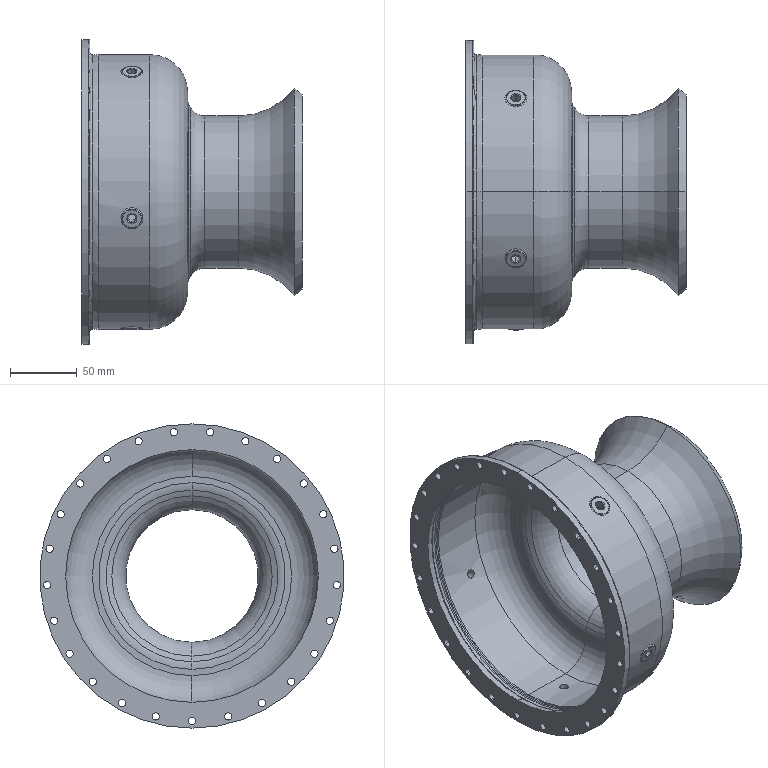Part | STEP file | Completa.sldasm-Part-25_Valor predeterminado | 1 solid | 173 faces | box 164.604 x 227.494 x 227.494 mm | volume 716979 mm3 | cylinder 77 | torus 54 | spline 25 | plane 9 | cone 4 | other 4 | commonest cylinder face diameters 5.4 x50 6.5 x10 14.5 x5 99.22 x2 113.714 x2 191 x2